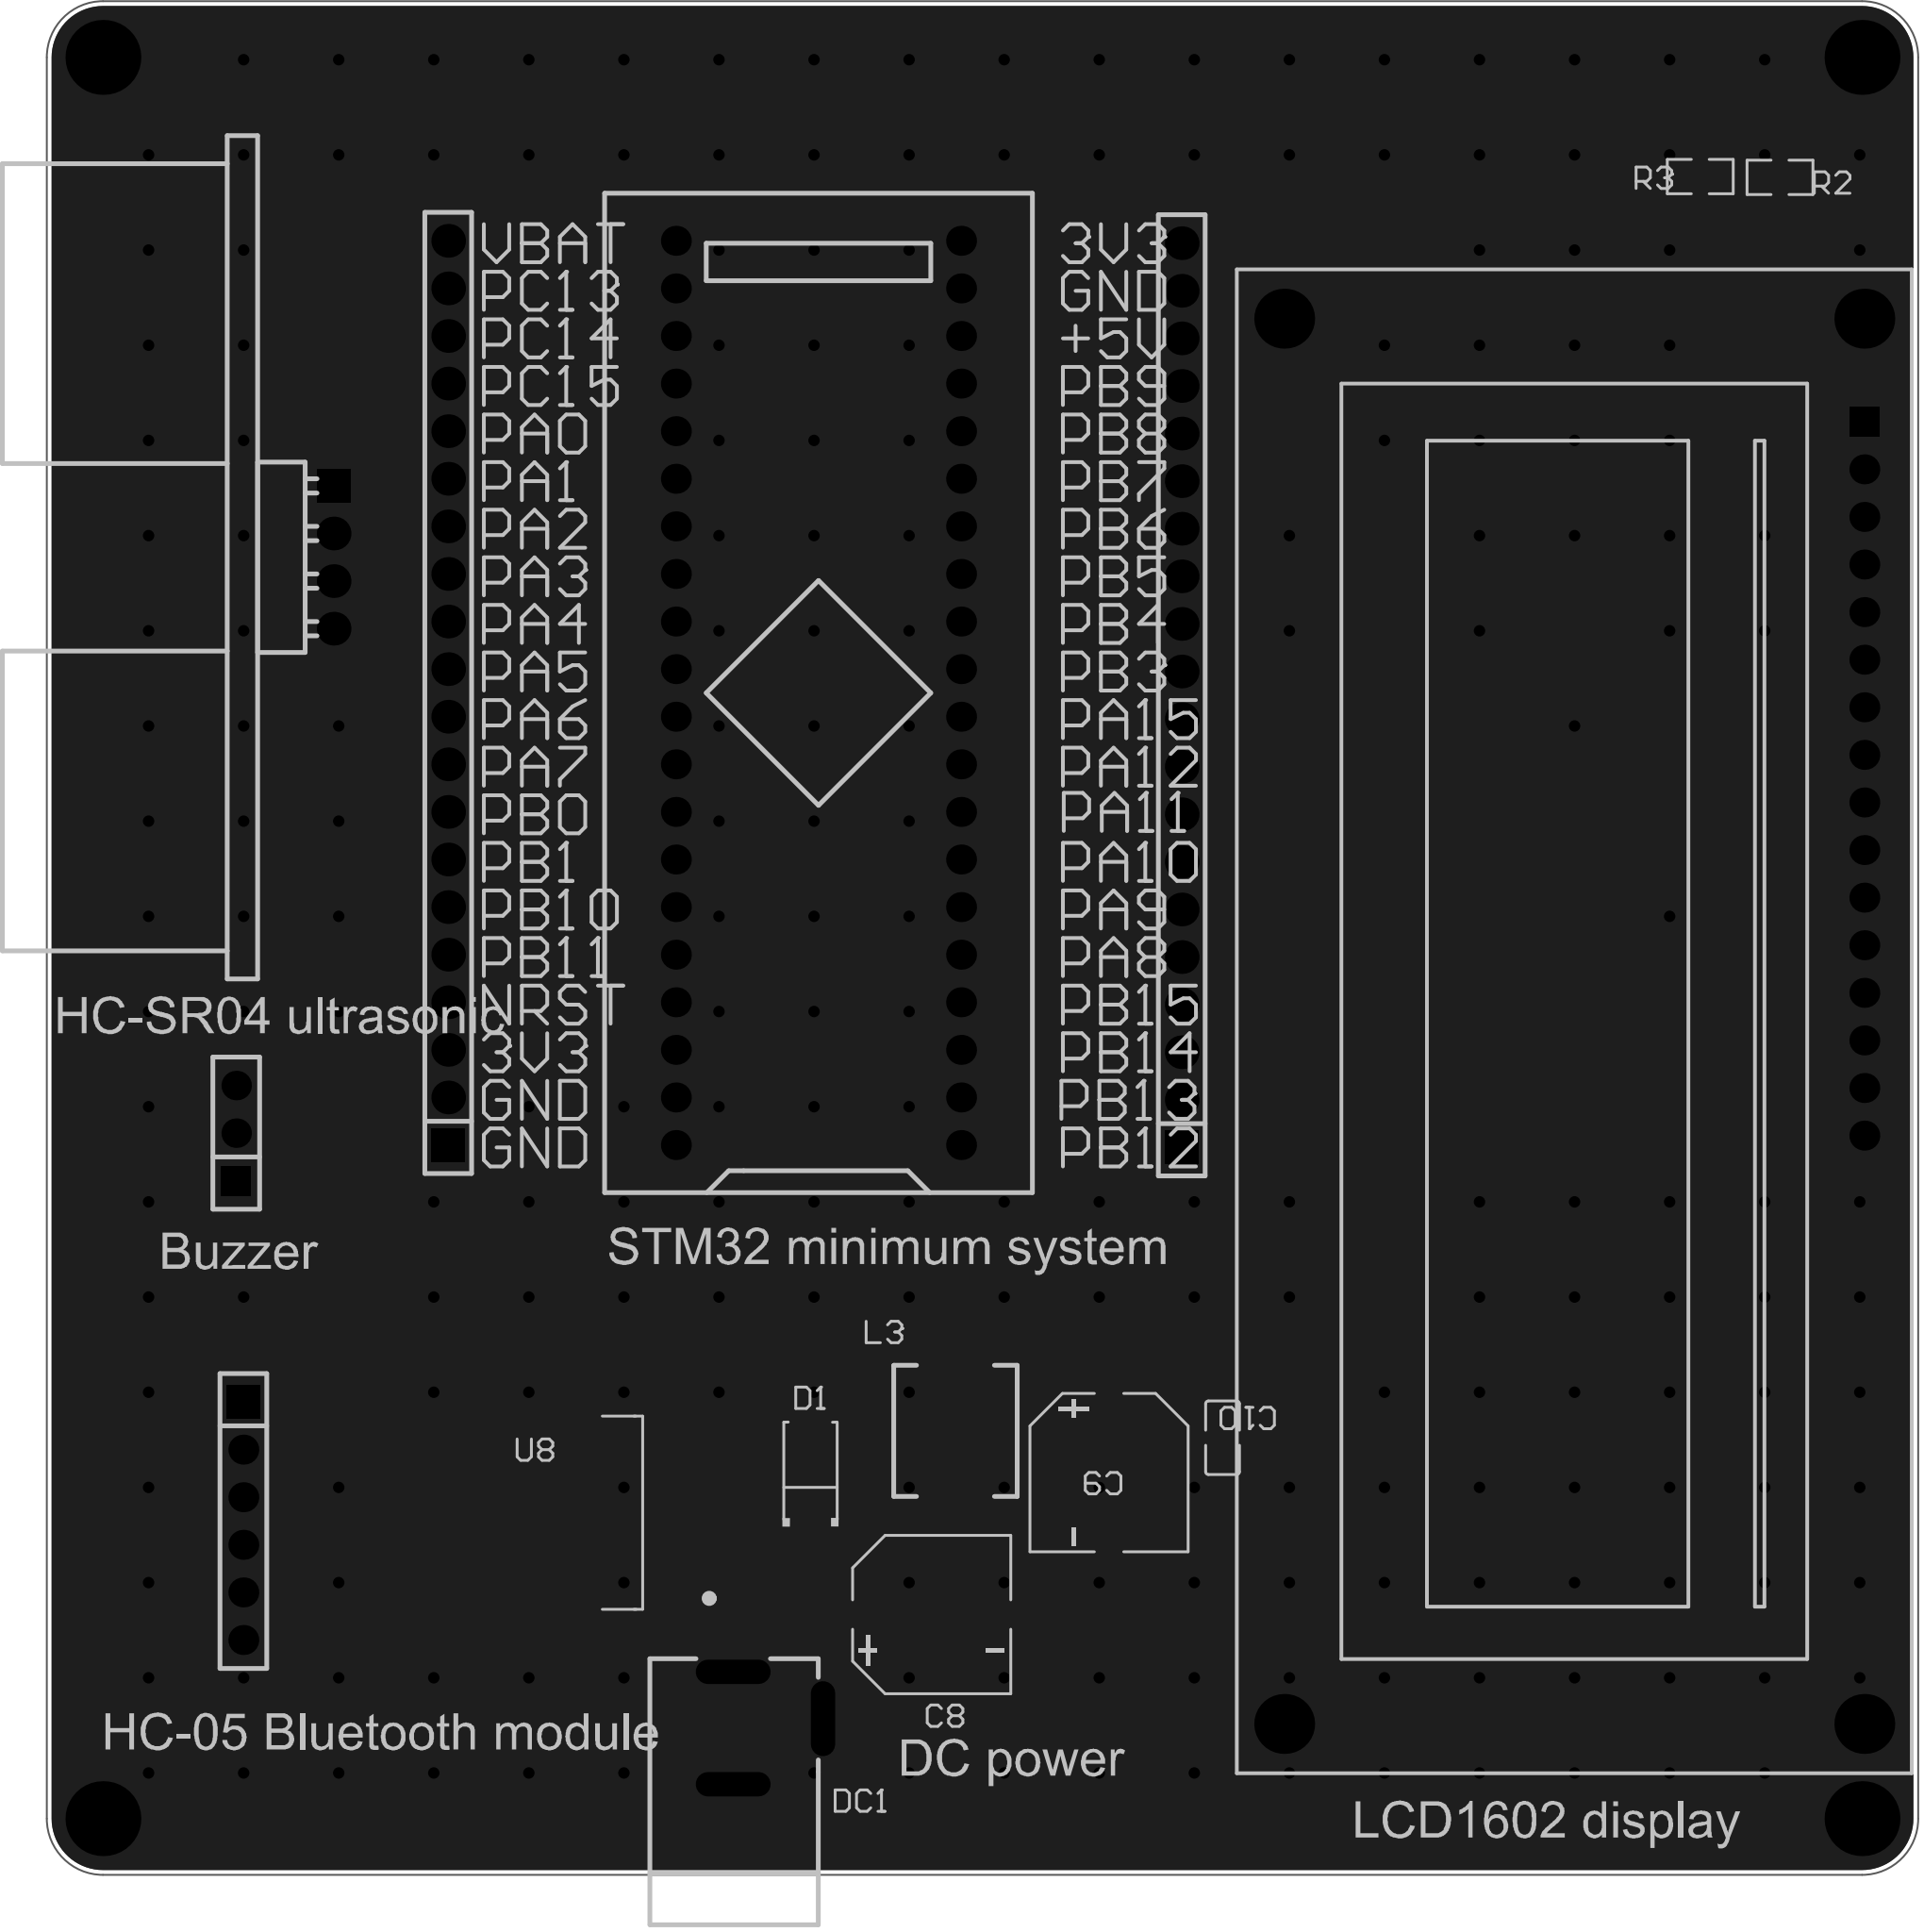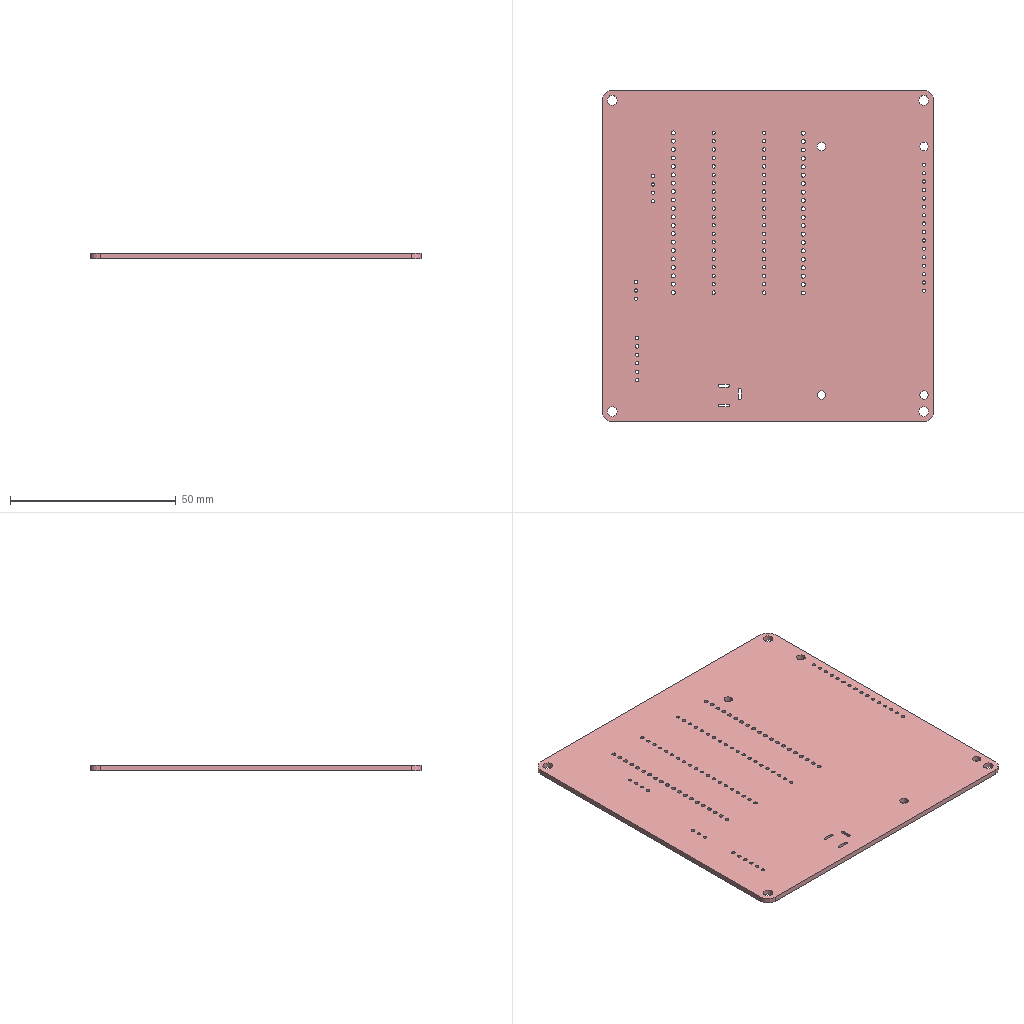Circuit board layout | Altium Designer | box 100 x 100 x 1.6 mm
Layer stack:
# Altium Designer layer stack of  (unit mm; dielectric type: 0 none, 1 core, 2 prepreg, 3 surface material)
index,name,kind,layer,copper_thickness_mm,dielectric_type,dielectric_thickness_mm,dielectric_material,dielectric_constant
0,Top Paste Mask Layer,other,,,,,,
1,Top Silkscreen Layer,other,,,,,,
2,Top Solder Mask Layer,dielectric,,,3,0.01,,3.3
3,Top Layer,copper,Top Layer,0.035,,,,
4,Dielectric1,dielectric,,,3,1.51,FR4,4.5
5,Bottom Layer,copper,Bottom Layer,0.035,,,,
6,Bottom Solder Mask Layer,dielectric,,,3,0.01,,3.3
7,Bottom Silkscreen Layer,other,,,,,,
8,Bottom Paste Mask Layer,other,,,,,,
# drill layer pairs: low layer,high layer
drill_pair,Top Layer,Bottom Layer
Part placement:
Designator,Comment,Layer,Footprint,Center-X(mm),Center-Y(mm),Rotation
U1,STM32F103C8T6-Card,TopLayer,CONN-TH_L53.3-W22.9_STM32F103C8T6-CARD,121.793,141.986,90
H1,,TopLayer,HDR-TH_20P-P2.54-V-F,141.203,141.859,90
H2,,TopLayer,HDR-TH_20P-P2.54-V-F,102.005,141.986,90
H3,,TopLayer,HDR-TH_6P-P2.54-V-F,91.059,97.79,270
H4,,TopLayer,HDR-TH_3P-P2.54-V-F,90.678,118.491,90
LCD1,LMB162ADC,TopLayer,LCD1602,162.179,124.46,270
R2,10K,TopLayer,R0805,173.171,169.502,0
R3,1K,TopLayer,R0805,168.91,169.545,0
U2,HC-SR04,TopLayer,TH_HC-SR04V,95.885,149.225,270
U8,LM2596S-5.0,TopLayer,TO-263-5_L10.2-W8.9-P1.70-BR,110.895,98.233,0
C10,,TopLayer,C0805,143.383,102.235,270
D1,,TopLayer,SMA_L4.3-W2.6-LS5.2-RD,121.364,100.469,90
C9,,TopLayer,CAP-SMD_BD8.0-L8.3-W8.3-RD,137.317,100.374,90
C8,,TopLayer,CAP-SMD_BD8.0-L8.3-W8.3-RD,127.841,92.798,180
L3,,TopLayer,IND-SMD_L7.0-W6.6,129.111,102.602,90
DC1,,TopLayer,DC-2.0,119.634,86.741,270
Pad and via stacks:
# Altium Designer via and pad stacks of  (unit mm). Each distinct definition once, with the count of objects using it.
# via: kind,start_layer,end_layer,hole_mm,diameter_mm,mode(0 simple;1 top-mid-bottom;2 full stack),diameter_per_layer,count,example_net
# pad: kind,layer,hole_mm,hole_type(0 round;1 square;2 slot),plating,top_size,top_shape(1 round;2 rect;3 octagon;9 rounded rect),mid_size,bottom_size,mode,footprint,size_per_layer,count,example
pad,Multi-Layer,3,0,plated,4x4,1,4x4,4x4,0,,,4,1
pad,Multi-Layer,1,0,plated,1.6x1.6,1,1.6x1.6,1.6x1.6,0,CONN-TH_L53.3-W22.9_STM32F103C8T6-CARD,,40,U1.1
pad,Multi-Layer,1.2,0,plated,1.8x1.8,2,1.8x1.8,1.8x1.8,0,HDR-TH_20P-P2.54-V-F,,2,H1.1
pad,Multi-Layer,1.2,0,plated,1.8x1.8,1,1.8x1.8,1.8x1.8,0,HDR-TH_20P-P2.54-V-F,,38,H1.2
pad,Multi-Layer,1.02,0,plated,1.6x1.6,1,1.6x1.6,1.6x1.6,0,HDR-TH_6P-P2.54-V-F,,5,H3.6
pad,Multi-Layer,1.02,0,plated,1.8x1.8,2,1.8x1.8,1.8x1.8,0,HDR-TH_6P-P2.54-V-F,,1,H3.1
pad,Multi-Layer,1.02,0,plated,1.575x1.575,1,1.575x1.575,1.575x1.575,0,HDR-TH_3P-P2.54-V-F,,2,H4.3
pad,Multi-Layer,1.02,0,plated,1.575x1.575,2,1.575x1.575,1.575x1.575,0,HDR-TH_3P-P2.54-V-F,,1,H4.1
pad,Multi-Layer,1,0,plated,1.6x1.6,1,1.6x1.6,1.6x1.6,0,LCD1602,,15,LCD1.16
pad,Multi-Layer,1,0,plated,1.6x1.6,2,1.6x1.6,1.6x1.6,0,LCD1602,,1,LCD1.1
pad,Multi-Layer,2.5,2,plated,3.2x3.2,1,3.2x3.2,3.2x3.2,0,LCD1602,,4,LCD1.0
pad,Multi-Layer,1.001,0,plated,1.8x1.8,1,1.8x1.8,1.8x1.8,0,TH_HC-SR04V,,3,U2.4
pad,Multi-Layer,1.001,0,plated,1.8x1.8,2,1.8x1.8,1.8x1.8,0,TH_HC-SR04V,,1,U2.1
pad,Multi-Layer,0.8001,2,plated,4x1.3,1,4x1.3,4x1.3,0,DC-2.0,,3,DC1.2
pad,Top Layer,0,0,plated,1.133x1.377,2,1.133x1.377,1.133x1.377,0,R0805,,4,R2.2
pad,Top Layer,0,0,plated,3.083x1.02,2,3.083x1.02,3.083x1.02,0,TO-263-5_L10.2-W8.9-P1.70-BR,,5,U8.1
pad,Top Layer,0,0,plated,8.5x11,2,8.5x11,8.5x11,0,TO-263-5_L10.2-W8.9-P1.70-BR,,1,U8.6
pad,Top Layer,0,0,plated,1.41x1.35,2,1.41x1.35,1.41x1.35,0,C0805,,2,C10.2
pad,Top Layer,0,0,plated,2x2,2,2x2,2x2,0,SMA_L4.3-W2.6-LS5.2-RD,,2,D1.2
pad,Top Layer,0,0,plated,3.61x1.26,2,3.61x1.26,3.61x1.26,0,CAP-SMD_BD8.0-L8.3-W8.3-RD,,4,C9.1
pad,Top Layer,0,0,plated,2.799x3.701,2,2.799x3.701,2.799x3.701,0,IND-SMD_L7.0-W6.6,,2,L3.1
via,Top Layer,Bottom Layer,0.3048,0.61,0,,222,GND
Copper pours:
name,layer,net,type(0 solid;1 hatched;2 none)
Bottom Layer-GND,Bottom Layer,GND,0
Top Layer-GND,Top Layer,GND,0